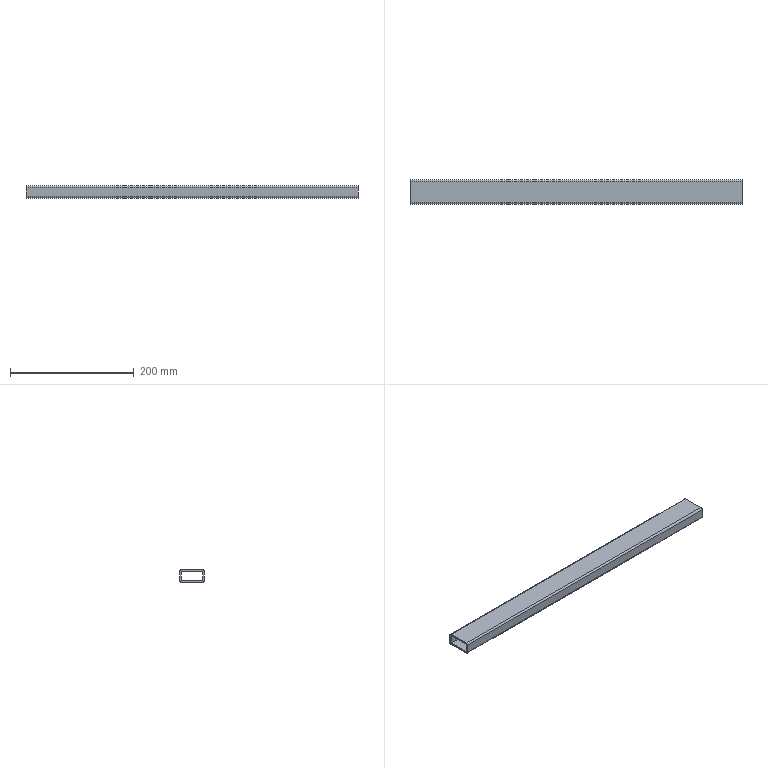Part | NX | features solid 2 | 1 solid | 28 faces | box 536 x 40 x 20 mm | volume 159680 mm3 | plane 24 | cylinder 4 | commonest cylinder face diameters 5.6 x4
STEP:
#1=CARTESIAN_POINT('',(-268.,-7.8,-847.));
#2=VERTEX_POINT('',#1);
#3=CARTESIAN_POINT('',(-268.,-42.2,-847.));
#4=VERTEX_POINT('',#3);
#5=CARTESIAN_POINT('',(-268.,-7.8,-847.));
#6=DIRECTION('',(0.,-1.,0.));
#7=VECTOR('',#6,1000.);
#8=LINE('',#5,#7);
#9=EDGE_CURVE('',#2,#4,#8,.T.);
#10=ORIENTED_EDGE('',*,*,#9,.T.);
#11=CARTESIAN_POINT('',(268.,-42.2,-847.));
#12=VERTEX_POINT('',#11);
#13=CARTESIAN_POINT('',(-268.,-42.2,-847.));
#14=DIRECTION('',(1.,0.,0.));
#15=VECTOR('',#14,1000.);
#16=LINE('',#13,#15);
#17=EDGE_CURVE('',#4,#12,#16,.T.);
#18=ORIENTED_EDGE('',*,*,#17,.T.);
#19=CARTESIAN_POINT('',(268.,-7.8,-847.));
#20=VERTEX_POINT('',#19);
#21=CARTESIAN_POINT('',(268.,-7.8,-847.));
#22=DIRECTION('',(0.,-1.,0.));
#23=VECTOR('',#22,1000.);
#24=LINE('',#21,#23);
#25=EDGE_CURVE('',#20,#12,#24,.T.);
#26=ORIENTED_EDGE('',*,*,#25,.F.);
#27=CARTESIAN_POINT('',(268.,-7.8,-847.));
#28=DIRECTION('',(-1.,0.,0.));
#29=VECTOR('',#28,1000.);
#30=LINE('',#27,#29);
#31=EDGE_CURVE('',#20,#2,#30,.T.);
#32=ORIENTED_EDGE('',*,*,#31,.T.);
#33=EDGE_LOOP('',(#10,#18,#26,#32));
#34=FACE_BOUND('',#33,.T.);
#35=CARTESIAN_POINT('',(-268.,-5.,-847.));
#36=DIRECTION('',(0.,0.,1.));
#37=DIRECTION('',(0.,1.,0.));
#38=AXIS2_PLACEMENT_3D('',#35,#36,#37);
#39=PLANE('',#38);
#40=ADVANCED_FACE('',(#34),#39,.T.);
#41=CARTESIAN_POINT('',(-268.,-5.,-849.8));
#42=VERTEX_POINT('',#41);
#43=CARTESIAN_POINT('',(-268.,-7.8,-849.8));
#44=DIRECTION('',(1.,0.,0.));
#45=DIRECTION('',(0.,1.,0.));
#46=AXIS2_PLACEMENT_3D('',#43,#44,#45);
#47=CIRCLE('',#46,2.8);
#48=EDGE_CURVE('',#42,#2,#47,.T.);
#49=ORIENTED_EDGE('',*,*,#48,.T.);
#50=ORIENTED_EDGE('',*,*,#31,.F.);
#51=CARTESIAN_POINT('',(268.,-5.,-849.8));
#52=VERTEX_POINT('',#51);
#53=CARTESIAN_POINT('',(268.,-7.8,-849.8));
#54=DIRECTION('',(-1.,0.,0.));
#55=DIRECTION('',(0.,0.,1.));
#56=AXIS2_PLACEMENT_3D('',#53,#54,#55);
#57=CIRCLE('',#56,2.8);
#58=EDGE_CURVE('',#20,#52,#57,.T.);
#59=ORIENTED_EDGE('',*,*,#58,.T.);
#60=CARTESIAN_POINT('',(-268.,-5.,-849.8));
#61=DIRECTION('',(1.,0.,0.));
#62=VECTOR('',#61,1000.);
#63=LINE('',#60,#62);
#64=EDGE_CURVE('',#42,#52,#63,.T.);
#65=ORIENTED_EDGE('',*,*,#64,.F.);
#66=EDGE_LOOP('',(#49,#50,#59,#65));
#67=FACE_BOUND('',#66,.T.);
#68=CARTESIAN_POINT('',(966.73,-7.8,-849.8));
#69=DIRECTION('',(-1.,0.,0.));
#70=DIRECTION('',(0.,0.,-1.));
#71=AXIS2_PLACEMENT_3D('',#68,#69,#70);
#72=CYLINDRICAL_SURFACE('',#71,2.8);
#73=ADVANCED_FACE('',(#67),#72,.T.);
#74=CARTESIAN_POINT('',(268.,-5.,-864.2));
#75=VERTEX_POINT('',#74);
#76=CARTESIAN_POINT('',(268.,-5.,-864.2));
#77=DIRECTION('',(0.,0.,1.));
#78=VECTOR('',#77,1000.);
#79=LINE('',#76,#78);
#80=EDGE_CURVE('',#75,#52,#79,.T.);
#81=ORIENTED_EDGE('',*,*,#80,.F.);
#82=CARTESIAN_POINT('',(-268.,-5.,-864.2));
#83=VERTEX_POINT('',#82);
#84=CARTESIAN_POINT('',(268.,-5.,-864.2));
#85=DIRECTION('',(-1.,0.,0.));
#86=VECTOR('',#85,1000.);
#87=LINE('',#84,#86);
#88=EDGE_CURVE('',#75,#83,#87,.T.);
#89=ORIENTED_EDGE('',*,*,#88,.T.);
#90=CARTESIAN_POINT('',(-268.,-5.,-864.2));
#91=DIRECTION('',(0.,0.,1.));
#92=VECTOR('',#91,1000.);
#93=LINE('',#90,#92);
#94=EDGE_CURVE('',#83,#42,#93,.T.);
#95=ORIENTED_EDGE('',*,*,#94,.T.);
#96=ORIENTED_EDGE('',*,*,#64,.T.);
#97=EDGE_LOOP('',(#81,#89,#95,#96));
#98=FACE_BOUND('',#97,.T.);
#99=CARTESIAN_POINT('',(-268.,-5.,-867.));
#100=DIRECTION('',(0.,1.,0.));
#101=DIRECTION('',(0.,0.,-1.));
#102=AXIS2_PLACEMENT_3D('',#99,#100,#101);
#103=PLANE('',#102);
#104=ADVANCED_FACE('',(#98),#103,.T.);
#105=ORIENTED_EDGE('',*,*,#94,.F.);
#106=CARTESIAN_POINT('',(-268.,-7.8,-864.2));
#107=VERTEX_POINT('',#106);
#108=CARTESIAN_POINT('',(-268.,-5.,-864.2));
#109=DIRECTION('',(0.,-1.,0.));
#110=VECTOR('',#109,1000.);
#111=LINE('',#108,#110);
#112=EDGE_CURVE('',#83,#107,#111,.T.);
#113=ORIENTED_EDGE('',*,*,#112,.T.);
#114=CARTESIAN_POINT('',(-268.,-7.8,-849.8));
#115=VERTEX_POINT('',#114);
#116=CARTESIAN_POINT('',(-268.,-7.8,-864.2));
#117=DIRECTION('',(0.,0.,1.));
#118=VECTOR('',#117,1000.);
#119=LINE('',#116,#118);
#120=EDGE_CURVE('',#107,#115,#119,.T.);
#121=ORIENTED_EDGE('',*,*,#120,.T.);
#122=CARTESIAN_POINT('',(-268.,-5.,-849.8));
#123=DIRECTION('',(0.,-1.,0.));
#124=VECTOR('',#123,1000.);
#125=LINE('',#122,#124);
#126=EDGE_CURVE('',#42,#115,#125,.T.);
#127=ORIENTED_EDGE('',*,*,#126,.F.);
#128=EDGE_LOOP('',(#105,#113,#121,#127));
#129=FACE_BOUND('',#128,.T.);
#130=CARTESIAN_POINT('',(-268.,-6.4,-857.));
#131=DIRECTION('',(-1.,0.,0.));
#132=DIRECTION('',(0.,0.,-1.));
#133=AXIS2_PLACEMENT_3D('',#130,#131,#132);
#134=PLANE('',#133);
#135=ADVANCED_FACE('',(#129),#134,.T.);
#136=ORIENTED_EDGE('',*,*,#126,.T.);
#137=CARTESIAN_POINT('',(-268.,-7.8,-847.));
#138=DIRECTION('',(0.,0.,-1.));
#139=VECTOR('',#138,1000.);
#140=LINE('',#137,#139);
#141=EDGE_CURVE('',#2,#115,#140,.T.);
#142=ORIENTED_EDGE('',*,*,#141,.F.);
#143=ORIENTED_EDGE('',*,*,#48,.F.);
#144=EDGE_LOOP('',(#136,#142,#143));
#145=FACE_BOUND('',#144,.T.);
#146=CARTESIAN_POINT('',(-268.,-6.81,-848.81));
#147=DIRECTION('',(1.,0.,0.));
#148=DIRECTION('',(0.,-1.,0.));
#149=AXIS2_PLACEMENT_3D('',#146,#147,#148);
#150=PLANE('',#149);
#151=ADVANCED_FACE('',(#145),#150,.F.);
#152=ORIENTED_EDGE('',*,*,#9,.F.);
#153=ORIENTED_EDGE('',*,*,#141,.T.);
#154=CARTESIAN_POINT('',(-268.,-42.2,-849.8));
#155=VERTEX_POINT('',#154);
#156=CARTESIAN_POINT('',(-268.,-7.8,-849.8));
#157=DIRECTION('',(0.,-1.,0.));
#158=VECTOR('',#157,1000.);
#159=LINE('',#156,#158);
#160=EDGE_CURVE('',#115,#155,#159,.T.);
#161=ORIENTED_EDGE('',*,*,#160,.T.);
#162=CARTESIAN_POINT('',(-268.,-42.2,-847.));
#163=DIRECTION('',(0.,0.,-1.));
#164=VECTOR('',#163,1000.);
#165=LINE('',#162,#164);
#166=EDGE_CURVE('',#4,#155,#165,.T.);
#167=ORIENTED_EDGE('',*,*,#166,.F.);
#168=EDGE_LOOP('',(#152,#153,#161,#167));
#169=FACE_BOUND('',#168,.T.);
#170=CARTESIAN_POINT('',(-268.,-25.,-848.4));
#171=DIRECTION('',(-1.,0.,0.));
#172=DIRECTION('',(0.,1.,0.));
#173=AXIS2_PLACEMENT_3D('',#170,#171,#172);
#174=PLANE('',#173);
#175=ADVANCED_FACE('',(#169),#174,.T.);
#176=ORIENTED_EDGE('',*,*,#166,.T.);
#177=CARTESIAN_POINT('',(-268.,-45.,-849.8));
#178=VERTEX_POINT('',#177);
#179=CARTESIAN_POINT('',(-268.,-45.,-849.8));
#180=DIRECTION('',(0.,1.,0.));
#181=VECTOR('',#180,1000.);
#182=LINE('',#179,#181);
#183=EDGE_CURVE('',#178,#155,#182,.T.);
#184=ORIENTED_EDGE('',*,*,#183,.F.);
#185=CARTESIAN_POINT('',(-268.,-42.2,-849.8));
#186=DIRECTION('',(1.,0.,0.));
#187=DIRECTION('',(0.,0.,1.));
#188=AXIS2_PLACEMENT_3D('',#185,#186,#187);
#189=CIRCLE('',#188,2.8);
#190=EDGE_CURVE('',#4,#178,#189,.T.);
#191=ORIENTED_EDGE('',*,*,#190,.F.);
#192=EDGE_LOOP('',(#176,#184,#191));
#193=FACE_BOUND('',#192,.T.);
#194=CARTESIAN_POINT('',(-268.,-43.19,-848.81));
#195=DIRECTION('',(1.,0.,0.));
#196=DIRECTION('',(0.,0.,-1.));
#197=AXIS2_PLACEMENT_3D('',#194,#195,#196);
#198=PLANE('',#197);
#199=ADVANCED_FACE('',(#193),#198,.F.);
#200=ORIENTED_EDGE('',*,*,#190,.T.);
#201=CARTESIAN_POINT('',(268.,-45.,-849.8));
#202=VERTEX_POINT('',#201);
#203=CARTESIAN_POINT('',(268.,-45.,-849.8));
#204=DIRECTION('',(-1.,0.,0.));
#205=VECTOR('',#204,1000.);
#206=LINE('',#203,#205);
#207=EDGE_CURVE('',#202,#178,#206,.T.);
#208=ORIENTED_EDGE('',*,*,#207,.F.);
#209=CARTESIAN_POINT('',(268.,-42.2,-849.8));
#210=DIRECTION('',(-1.,0.,0.));
#211=DIRECTION('',(0.,-1.,0.));
#212=AXIS2_PLACEMENT_3D('',#209,#210,#211);
#213=CIRCLE('',#212,2.8);
#214=EDGE_CURVE('',#202,#12,#213,.T.);
#215=ORIENTED_EDGE('',*,*,#214,.T.);
#216=ORIENTED_EDGE('',*,*,#17,.F.);
#217=EDGE_LOOP('',(#200,#208,#215,#216));
#218=FACE_BOUND('',#217,.T.);
#219=CARTESIAN_POINT('',(966.73,-42.2,-849.8));
#220=DIRECTION('',(-1.,0.,0.));
#221=DIRECTION('',(0.,1.,0.));
#222=AXIS2_PLACEMENT_3D('',#219,#220,#221);
#223=CYLINDRICAL_SURFACE('',#222,2.8);
#224=ADVANCED_FACE('',(#218),#223,.T.);
#225=CARTESIAN_POINT('',(268.,-42.2,-849.8));
#226=VERTEX_POINT('',#225);
#227=CARTESIAN_POINT('',(268.,-45.,-849.8));
#228=DIRECTION('',(0.,1.,0.));
#229=VECTOR('',#228,1000.);
#230=LINE('',#227,#229);
#231=EDGE_CURVE('',#202,#226,#230,.T.);
#232=ORIENTED_EDGE('',*,*,#231,.T.);
#233=CARTESIAN_POINT('',(268.,-42.2,-847.));
#234=DIRECTION('',(0.,0.,-1.));
#235=VECTOR('',#234,1000.);
#236=LINE('',#233,#235);
#237=EDGE_CURVE('',#12,#226,#236,.T.);
#238=ORIENTED_EDGE('',*,*,#237,.F.);
#239=ORIENTED_EDGE('',*,*,#214,.F.);
#240=EDGE_LOOP('',(#232,#238,#239));
#241=FACE_BOUND('',#240,.T.);
#242=CARTESIAN_POINT('',(268.,-43.19,-848.81));
#243=DIRECTION('',(-1.,0.,0.));
#244=DIRECTION('',(0.,1.,0.));
#245=AXIS2_PLACEMENT_3D('',#242,#243,#244);
#246=PLANE('',#245);
#247=ADVANCED_FACE('',(#241),#246,.F.);
#248=ORIENTED_EDGE('',*,*,#25,.T.);
#249=ORIENTED_EDGE('',*,*,#237,.T.);
#250=CARTESIAN_POINT('',(268.,-7.8,-849.8));
#251=VERTEX_POINT('',#250);
#252=CARTESIAN_POINT('',(268.,-7.8,-849.8));
#253=DIRECTION('',(0.,-1.,0.));
#254=VECTOR('',#253,1000.);
#255=LINE('',#252,#254);
#256=EDGE_CURVE('',#251,#226,#255,.T.);
#257=ORIENTED_EDGE('',*,*,#256,.F.);
#258=CARTESIAN_POINT('',(268.,-7.8,-847.));
#259=DIRECTION('',(0.,0.,-1.));
#260=VECTOR('',#259,1000.);
#261=LINE('',#258,#260);
#262=EDGE_CURVE('',#20,#251,#261,.T.);
#263=ORIENTED_EDGE('',*,*,#262,.F.);
#264=EDGE_LOOP('',(#248,#249,#257,#263));
#265=FACE_BOUND('',#264,.T.);
#266=CARTESIAN_POINT('',(268.,-25.,-848.4));
#267=DIRECTION('',(-1.,0.,0.));
#268=DIRECTION('',(0.,1.,0.));
#269=AXIS2_PLACEMENT_3D('',#266,#267,#268);
#270=PLANE('',#269);
#271=ADVANCED_FACE('',(#265),#270,.F.);
#272=ORIENTED_EDGE('',*,*,#262,.T.);
#273=CARTESIAN_POINT('',(268.,-5.,-849.8));
#274=DIRECTION('',(0.,-1.,0.));
#275=VECTOR('',#274,1000.);
#276=LINE('',#273,#275);
#277=EDGE_CURVE('',#52,#251,#276,.T.);
#278=ORIENTED_EDGE('',*,*,#277,.F.);
#279=ORIENTED_EDGE('',*,*,#58,.F.);
#280=EDGE_LOOP('',(#272,#278,#279));
#281=FACE_BOUND('',#280,.T.);
#282=CARTESIAN_POINT('',(268.,-6.81,-848.81));
#283=DIRECTION('',(-1.,0.,0.));
#284=DIRECTION('',(0.,0.,-1.));
#285=AXIS2_PLACEMENT_3D('',#282,#283,#284);
#286=PLANE('',#285);
#287=ADVANCED_FACE('',(#281),#286,.F.);
#288=ORIENTED_EDGE('',*,*,#80,.T.);
#289=ORIENTED_EDGE('',*,*,#277,.T.);
#290=CARTESIAN_POINT('',(268.,-7.8,-864.2));
#291=VERTEX_POINT('',#290);
#292=CARTESIAN_POINT('',(268.,-7.8,-864.2));
#293=DIRECTION('',(0.,0.,1.));
#294=VECTOR('',#293,1000.);
#295=LINE('',#292,#294);
#296=EDGE_CURVE('',#291,#251,#295,.T.);
#297=ORIENTED_EDGE('',*,*,#296,.F.);
#298=CARTESIAN_POINT('',(268.,-5.,-864.2));
#299=DIRECTION('',(0.,-1.,0.));
#300=VECTOR('',#299,1000.);
#301=LINE('',#298,#300);
#302=EDGE_CURVE('',#75,#291,#301,.T.);
#303=ORIENTED_EDGE('',*,*,#302,.F.);
#304=EDGE_LOOP('',(#288,#289,#297,#303));
#305=FACE_BOUND('',#304,.T.);
#306=CARTESIAN_POINT('',(268.,-6.4,-857.));
#307=DIRECTION('',(-1.,0.,0.));
#308=DIRECTION('',(0.,0.,-1.));
#309=AXIS2_PLACEMENT_3D('',#306,#307,#308);
#310=PLANE('',#309);
#311=ADVANCED_FACE('',(#305),#310,.F.);
#312=ORIENTED_EDGE('',*,*,#302,.T.);
#313=CARTESIAN_POINT('',(268.,-7.8,-867.));
#314=VERTEX_POINT('',#313);
#315=CARTESIAN_POINT('',(268.,-7.8,-867.));
#316=DIRECTION('',(0.,0.,1.));
#317=VECTOR('',#316,1000.);
#318=LINE('',#315,#317);
#319=EDGE_CURVE('',#314,#291,#318,.T.);
#320=ORIENTED_EDGE('',*,*,#319,.F.);
#321=CARTESIAN_POINT('',(268.,-7.8,-864.2));
#322=DIRECTION('',(-1.,0.,0.));
#323=DIRECTION('',(0.,1.,0.));
#324=AXIS2_PLACEMENT_3D('',#321,#322,#323);
#325=CIRCLE('',#324,2.8);
#326=EDGE_CURVE('',#75,#314,#325,.T.);
#327=ORIENTED_EDGE('',*,*,#326,.F.);
#328=EDGE_LOOP('',(#312,#320,#327));
#329=FACE_BOUND('',#328,.T.);
#330=CARTESIAN_POINT('',(268.,-6.81,-865.19));
#331=DIRECTION('',(-1.,0.,0.));
#332=DIRECTION('',(0.,-1.,0.));
#333=AXIS2_PLACEMENT_3D('',#330,#331,#332);
#334=PLANE('',#333);
#335=ADVANCED_FACE('',(#329),#334,.F.);
#336=CARTESIAN_POINT('',(-268.,-7.8,-867.));
#337=VERTEX_POINT('',#336);
#338=CARTESIAN_POINT('',(-268.,-7.8,-864.2));
#339=DIRECTION('',(1.,0.,0.));
#340=DIRECTION('',(0.,0.,-1.));
#341=AXIS2_PLACEMENT_3D('',#338,#339,#340);
#342=CIRCLE('',#341,2.8);
#343=EDGE_CURVE('',#337,#83,#342,.T.);
#344=ORIENTED_EDGE('',*,*,#343,.T.);
#345=ORIENTED_EDGE('',*,*,#88,.F.);
#346=ORIENTED_EDGE('',*,*,#326,.T.);
#347=CARTESIAN_POINT('',(-268.,-7.8,-867.));
#348=DIRECTION('',(1.,0.,0.));
#349=VECTOR('',#348,1000.);
#350=LINE('',#347,#349);
#351=EDGE_CURVE('',#337,#314,#350,.T.);
#352=ORIENTED_EDGE('',*,*,#351,.F.);
#353=EDGE_LOOP('',(#344,#345,#346,#352));
#354=FACE_BOUND('',#353,.T.);
#355=CARTESIAN_POINT('',(966.73,-7.8,-864.2));
#356=DIRECTION('',(-1.,0.,0.));
#357=DIRECTION('',(0.,-1.,0.));
#358=AXIS2_PLACEMENT_3D('',#355,#356,#357);
#359=CYLINDRICAL_SURFACE('',#358,2.8);
#360=ADVANCED_FACE('',(#354),#359,.T.);
#361=CARTESIAN_POINT('',(268.,-42.2,-867.));
#362=VERTEX_POINT('',#361);
#363=CARTESIAN_POINT('',(268.,-42.2,-867.));
#364=DIRECTION('',(0.,1.,0.));
#365=VECTOR('',#364,1000.);
#366=LINE('',#363,#365);
#367=EDGE_CURVE('',#362,#314,#366,.T.);
#368=ORIENTED_EDGE('',*,*,#367,.F.);
#369=CARTESIAN_POINT('',(-268.,-42.2,-867.));
#370=VERTEX_POINT('',#369);
#371=CARTESIAN_POINT('',(268.,-42.2,-867.));
#372=DIRECTION('',(-1.,0.,0.));
#373=VECTOR('',#372,1000.);
#374=LINE('',#371,#373);
#375=EDGE_CURVE('',#362,#370,#374,.T.);
#376=ORIENTED_EDGE('',*,*,#375,.T.);
#377=CARTESIAN_POINT('',(-268.,-42.2,-867.));
#378=DIRECTION('',(0.,1.,0.));
#379=VECTOR('',#378,1000.);
#380=LINE('',#377,#379);
#381=EDGE_CURVE('',#370,#337,#380,.T.);
#382=ORIENTED_EDGE('',*,*,#381,.T.);
#383=ORIENTED_EDGE('',*,*,#351,.T.);
#384=EDGE_LOOP('',(#368,#376,#382,#383));
#385=FACE_BOUND('',#384,.T.);
#386=CARTESIAN_POINT('',(-268.,-45.,-867.));
#387=DIRECTION('',(0.,0.,-1.));
#388=DIRECTION('',(0.,-1.,0.));
#389=AXIS2_PLACEMENT_3D('',#386,#387,#388);
#390=PLANE('',#389);
#391=ADVANCED_FACE('',(#385),#390,.T.);
#392=ORIENTED_EDGE('',*,*,#381,.F.);
#393=CARTESIAN_POINT('',(-268.,-42.2,-864.2));
#394=VERTEX_POINT('',#393);
#395=CARTESIAN_POINT('',(-268.,-42.2,-867.));
#396=DIRECTION('',(0.,0.,1.));
#397=VECTOR('',#396,1000.);
#398=LINE('',#395,#397);
#399=EDGE_CURVE('',#370,#394,#398,.T.);
#400=ORIENTED_EDGE('',*,*,#399,.T.);
#401=CARTESIAN_POINT('',(-268.,-42.2,-864.2));
#402=DIRECTION('',(0.,1.,0.));
#403=VECTOR('',#402,1000.);
#404=LINE('',#401,#403);
#405=EDGE_CURVE('',#394,#107,#404,.T.);
#406=ORIENTED_EDGE('',*,*,#405,.T.);
#407=CARTESIAN_POINT('',(-268.,-7.8,-867.));
#408=DIRECTION('',(0.,0.,1.));
#409=VECTOR('',#408,1000.);
#410=LINE('',#407,#409);
#411=EDGE_CURVE('',#337,#107,#410,.T.);
#412=ORIENTED_EDGE('',*,*,#411,.F.);
#413=EDGE_LOOP('',(#392,#400,#406,#412));
#414=FACE_BOUND('',#413,.T.);
#415=CARTESIAN_POINT('',(-268.,-25.,-865.6));
#416=DIRECTION('',(-1.,0.,0.));
#417=DIRECTION('',(0.,-1.,0.));
#418=AXIS2_PLACEMENT_3D('',#415,#416,#417);
#419=PLANE('',#418);
#420=ADVANCED_FACE('',(#414),#419,.T.);
#421=ORIENTED_EDGE('',*,*,#411,.T.);
#422=ORIENTED_EDGE('',*,*,#112,.F.);
#423=ORIENTED_EDGE('',*,*,#343,.F.);
#424=EDGE_LOOP('',(#421,#422,#423));
#425=FACE_BOUND('',#424,.T.);
#426=CARTESIAN_POINT('',(-268.,-6.81,-865.19));
#427=DIRECTION('',(1.,0.,0.));
#428=DIRECTION('',(0.,0.,1.));
#429=AXIS2_PLACEMENT_3D('',#426,#427,#428);
#430=PLANE('',#429);
#431=ADVANCED_FACE('',(#425),#430,.F.);
#432=ORIENTED_EDGE('',*,*,#405,.F.);
#433=CARTESIAN_POINT('',(268.,-42.2,-864.2));
#434=VERTEX_POINT('',#433);
#435=CARTESIAN_POINT('',(268.,-42.2,-864.2));
#436=DIRECTION('',(-1.,0.,0.));
#437=VECTOR('',#436,1000.);
#438=LINE('',#435,#437);
#439=EDGE_CURVE('',#434,#394,#438,.T.);
#440=ORIENTED_EDGE('',*,*,#439,.F.);
#441=CARTESIAN_POINT('',(268.,-42.2,-864.2));
#442=DIRECTION('',(0.,1.,0.));
#443=VECTOR('',#442,1000.);
#444=LINE('',#441,#443);
#445=EDGE_CURVE('',#434,#291,#444,.T.);
#446=ORIENTED_EDGE('',*,*,#445,.T.);
#447=CARTESIAN_POINT('',(268.,-7.8,-864.2));
#448=DIRECTION('',(-1.,0.,0.));
#449=VECTOR('',#448,1000.);
#450=LINE('',#447,#449);
#451=EDGE_CURVE('',#291,#107,#450,.T.);
#452=ORIENTED_EDGE('',*,*,#451,.T.);
#453=EDGE_LOOP('',(#432,#440,#446,#452));
#454=FACE_BOUND('',#453,.T.);
#455=CARTESIAN_POINT('',(-268.,-45.,-864.2));
#456=DIRECTION('',(0.,0.,-1.));
#457=DIRECTION('',(0.,-1.,0.));
#458=AXIS2_PLACEMENT_3D('',#455,#456,#457);
#459=PLANE('',#458);
#460=ADVANCED_FACE('',(#454),#459,.F.);
#461=ORIENTED_EDGE('',*,*,#120,.F.);
#462=ORIENTED_EDGE('',*,*,#451,.F.);
#463=ORIENTED_EDGE('',*,*,#296,.T.);
#464=CARTESIAN_POINT('',(268.,-7.8,-849.8));
#465=DIRECTION('',(-1.,0.,0.));
#466=VECTOR('',#465,1000.);
#467=LINE('',#464,#466);
#468=EDGE_CURVE('',#251,#115,#467,.T.);
#469=ORIENTED_EDGE('',*,*,#468,.T.);
#470=EDGE_LOOP('',(#461,#462,#463,#469));
#471=FACE_BOUND('',#470,.T.);
#472=CARTESIAN_POINT('',(-268.,-7.8,-867.));
#473=DIRECTION('',(0.,1.,0.));
#474=DIRECTION('',(0.,0.,-1.));
#475=AXIS2_PLACEMENT_3D('',#472,#473,#474);
#476=PLANE('',#475);
#477=ADVANCED_FACE('',(#471),#476,.F.);
#478=ORIENTED_EDGE('',*,*,#256,.T.);
#479=CARTESIAN_POINT('',(268.,-42.2,-849.8));
#480=DIRECTION('',(-1.,0.,0.));
#481=VECTOR('',#480,1000.);
#482=LINE('',#479,#481);
#483=EDGE_CURVE('',#226,#155,#482,.T.);
#484=ORIENTED_EDGE('',*,*,#483,.T.);
#485=ORIENTED_EDGE('',*,*,#160,.F.);
#486=ORIENTED_EDGE('',*,*,#468,.F.);
#487=EDGE_LOOP('',(#478,#484,#485,#486));
#488=FACE_BOUND('',#487,.T.);
#489=CARTESIAN_POINT('',(-268.,-5.,-849.8));
#490=DIRECTION('',(0.,0.,1.));
#491=DIRECTION('',(0.,1.,0.));
#492=AXIS2_PLACEMENT_3D('',#489,#490,#491);
#493=PLANE('',#492);
#494=ADVANCED_FACE('',(#488),#493,.F.);
#495=CARTESIAN_POINT('',(268.,-42.2,-849.8));
#496=DIRECTION('',(0.,0.,-1.));
#497=VECTOR('',#496,1000.);
#498=LINE('',#495,#497);
#499=EDGE_CURVE('',#226,#434,#498,.T.);
#500=ORIENTED_EDGE('',*,*,#499,.T.);
#501=ORIENTED_EDGE('',*,*,#439,.T.);
#502=CARTESIAN_POINT('',(-268.,-42.2,-849.8));
#503=DIRECTION('',(0.,0.,-1.));
#504=VECTOR('',#503,1000.);
#505=LINE('',#502,#504);
#506=EDGE_CURVE('',#155,#394,#505,.T.);
#507=ORIENTED_EDGE('',*,*,#506,.F.);
#508=ORIENTED_EDGE('',*,*,#483,.F.);
#509=EDGE_LOOP('',(#500,#501,#507,#508));
#510=FACE_BOUND('',#509,.T.);
#511=CARTESIAN_POINT('',(-268.,-42.2,-847.));
#512=DIRECTION('',(0.,-1.,0.));
#513=DIRECTION('',(0.,0.,1.));
#514=AXIS2_PLACEMENT_3D('',#511,#512,#513);
#515=PLANE('',#514);
#516=ADVANCED_FACE('',(#510),#515,.F.);
#517=CARTESIAN_POINT('',(-268.,-45.,-864.2));
#518=VERTEX_POINT('',#517);
#519=CARTESIAN_POINT('',(-268.,-45.,-849.8));
#520=DIRECTION('',(0.,0.,-1.));
#521=VECTOR('',#520,1000.);
#522=LINE('',#519,#521);
#523=EDGE_CURVE('',#178,#518,#522,.T.);
#524=ORIENTED_EDGE('',*,*,#523,.F.);
#525=ORIENTED_EDGE('',*,*,#183,.T.);
#526=ORIENTED_EDGE('',*,*,#506,.T.);
#527=CARTESIAN_POINT('',(-268.,-45.,-864.2));
#528=DIRECTION('',(0.,1.,0.));
#529=VECTOR('',#528,1000.);
#530=LINE('',#527,#529);
#531=EDGE_CURVE('',#518,#394,#530,.T.);
#532=ORIENTED_EDGE('',*,*,#531,.F.);
#533=EDGE_LOOP('',(#524,#525,#526,#532));
#534=FACE_BOUND('',#533,.T.);
#535=CARTESIAN_POINT('',(-268.,-43.6,-857.));
#536=DIRECTION('',(-1.,0.,0.));
#537=DIRECTION('',(0.,0.,1.));
#538=AXIS2_PLACEMENT_3D('',#535,#536,#537);
#539=PLANE('',#538);
#540=ADVANCED_FACE('',(#534),#539,.T.);
#541=ORIENTED_EDGE('',*,*,#531,.T.);
#542=ORIENTED_EDGE('',*,*,#399,.F.);
#543=CARTESIAN_POINT('',(-268.,-42.2,-864.2));
#544=DIRECTION('',(1.,0.,0.));
#545=DIRECTION('',(0.,-1.,0.));
#546=AXIS2_PLACEMENT_3D('',#543,#544,#545);
#547=CIRCLE('',#546,2.8);
#548=EDGE_CURVE('',#518,#370,#547,.T.);
#549=ORIENTED_EDGE('',*,*,#548,.F.);
#550=EDGE_LOOP('',(#541,#542,#549));
#551=FACE_BOUND('',#550,.T.);
#552=CARTESIAN_POINT('',(-268.,-43.19,-865.19));
#553=DIRECTION('',(1.,0.,0.));
#554=DIRECTION('',(0.,1.,0.));
#555=AXIS2_PLACEMENT_3D('',#552,#553,#554);
#556=PLANE('',#555);
#557=ADVANCED_FACE('',(#551),#556,.F.);
#558=ORIENTED_EDGE('',*,*,#548,.T.);
#559=ORIENTED_EDGE('',*,*,#375,.F.);
#560=CARTESIAN_POINT('',(268.,-45.,-864.2));
#561=VERTEX_POINT('',#560);
#562=CARTESIAN_POINT('',(268.,-42.2,-864.2));
#563=DIRECTION('',(-1.,0.,0.));
#564=DIRECTION('',(0.,0.,-1.));
#565=AXIS2_PLACEMENT_3D('',#562,#563,#564);
#566=CIRCLE('',#565,2.8);
#567=EDGE_CURVE('',#362,#561,#566,.T.);
#568=ORIENTED_EDGE('',*,*,#567,.T.);
#569=CARTESIAN_POINT('',(-268.,-45.,-864.2));
#570=DIRECTION('',(1.,0.,0.));
#571=VECTOR('',#570,1000.);
#572=LINE('',#569,#571);
#573=EDGE_CURVE('',#518,#561,#572,.T.);
#574=ORIENTED_EDGE('',*,*,#573,.F.);
#575=EDGE_LOOP('',(#558,#559,#568,#574));
#576=FACE_BOUND('',#575,.T.);
#577=CARTESIAN_POINT('',(966.73,-42.2,-864.2));
#578=DIRECTION('',(-1.,0.,0.));
#579=DIRECTION('',(0.,0.,1.));
#580=AXIS2_PLACEMENT_3D('',#577,#578,#579);
#581=CYLINDRICAL_SURFACE('',#580,2.8);
#582=ADVANCED_FACE('',(#576),#581,.T.);
#583=ORIENTED_EDGE('',*,*,#523,.T.);
#584=ORIENTED_EDGE('',*,*,#573,.T.);
#585=CARTESIAN_POINT('',(268.,-45.,-849.8));
#586=DIRECTION('',(0.,0.,-1.));
#587=VECTOR('',#586,1000.);
#588=LINE('',#585,#587);
#589=EDGE_CURVE('',#202,#561,#588,.T.);
#590=ORIENTED_EDGE('',*,*,#589,.F.);
#591=ORIENTED_EDGE('',*,*,#207,.T.);
#592=EDGE_LOOP('',(#583,#584,#590,#591));
#593=FACE_BOUND('',#592,.T.);
#594=CARTESIAN_POINT('',(-268.,-45.,-847.));
#595=DIRECTION('',(0.,-1.,0.));
#596=DIRECTION('',(0.,0.,1.));
#597=AXIS2_PLACEMENT_3D('',#594,#595,#596);
#598=PLANE('',#597);
#599=ADVANCED_FACE('',(#593),#598,.T.);
#600=ORIENTED_EDGE('',*,*,#589,.T.);
#601=CARTESIAN_POINT('',(268.,-45.,-864.2));
#602=DIRECTION('',(0.,1.,0.));
#603=VECTOR('',#602,1000.);
#604=LINE('',#601,#603);
#605=EDGE_CURVE('',#561,#434,#604,.T.);
#606=ORIENTED_EDGE('',*,*,#605,.T.);
#607=ORIENTED_EDGE('',*,*,#499,.F.);
#608=ORIENTED_EDGE('',*,*,#231,.F.);
#609=EDGE_LOOP('',(#600,#606,#607,#608));
#610=FACE_BOUND('',#609,.T.);
#611=CARTESIAN_POINT('',(268.,-43.6,-857.));
#612=DIRECTION('',(-1.,0.,0.));
#613=DIRECTION('',(0.,0.,1.));
#614=AXIS2_PLACEMENT_3D('',#611,#612,#613);
#615=PLANE('',#614);
#616=ADVANCED_FACE('',(#610),#615,.F.);
#617=CARTESIAN_POINT('',(268.,-42.2,-867.));
#618=DIRECTION('',(0.,0.,1.));
#619=VECTOR('',#618,1000.);
#620=LINE('',#617,#619);
#621=EDGE_CURVE('',#362,#434,#620,.T.);
#622=ORIENTED_EDGE('',*,*,#621,.T.);
#623=ORIENTED_EDGE('',*,*,#605,.F.);
#624=ORIENTED_EDGE('',*,*,#567,.F.);
#625=EDGE_LOOP('',(#622,#623,#624));
#626=FACE_BOUND('',#625,.T.);
#627=CARTESIAN_POINT('',(268.,-43.19,-865.19));
#628=DIRECTION('',(-1.,0.,0.));
#629=DIRECTION('',(0.,0.,1.));
#630=AXIS2_PLACEMENT_3D('',#627,#628,#629);
#631=PLANE('',#630);
#632=ADVANCED_FACE('',(#626),#631,.F.);
#633=ORIENTED_EDGE('',*,*,#367,.T.);
#634=ORIENTED_EDGE('',*,*,#319,.T.);
#635=ORIENTED_EDGE('',*,*,#445,.F.);
#636=ORIENTED_EDGE('',*,*,#621,.F.);
#637=EDGE_LOOP('',(#633,#634,#635,#636));
#638=FACE_BOUND('',#637,.T.);
#639=CARTESIAN_POINT('',(268.,-25.,-865.6));
#640=DIRECTION('',(-1.,0.,0.));
#641=DIRECTION('',(0.,-1.,0.));
#642=AXIS2_PLACEMENT_3D('',#639,#640,#641);
#643=PLANE('',#642);
#644=ADVANCED_FACE('',(#638),#643,.F.);
#645=CLOSED_SHELL('',(#40,#73,#104,#135,#151,#175,#199,#224,#247,#271,#287,#311,#335,#360,#391,#420,#431,#460,#477,#494,#516,#540,#557,#582,#599,#616,#632,#644));
#646=MANIFOLD_SOLID_BREP('',#645);
#647=(LENGTH_UNIT()NAMED_UNIT(*)SI_UNIT(.MILLI.,.METRE.));
#648=UNCERTAINTY_MEASURE_WITH_UNIT(LENGTH_MEASURE(0.00001),#647,'','');
#649=(NAMED_UNIT(*)PLANE_ANGLE_UNIT()SI_UNIT($,.RADIAN.));
#650=(NAMED_UNIT(*)SI_UNIT($,.STERADIAN.)SOLID_ANGLE_UNIT());
#651=(GEOMETRIC_REPRESENTATION_CONTEXT(3)GLOBAL_UNCERTAINTY_ASSIGNED_CONTEXT((#648))GLOBAL_UNIT_ASSIGNED_CONTEXT((#647,#649,#650))REPRESENTATION_CONTEXT('',''));
#652=ADVANCED_BREP_SHAPE_REPRESENTATION('',(#646),#651);